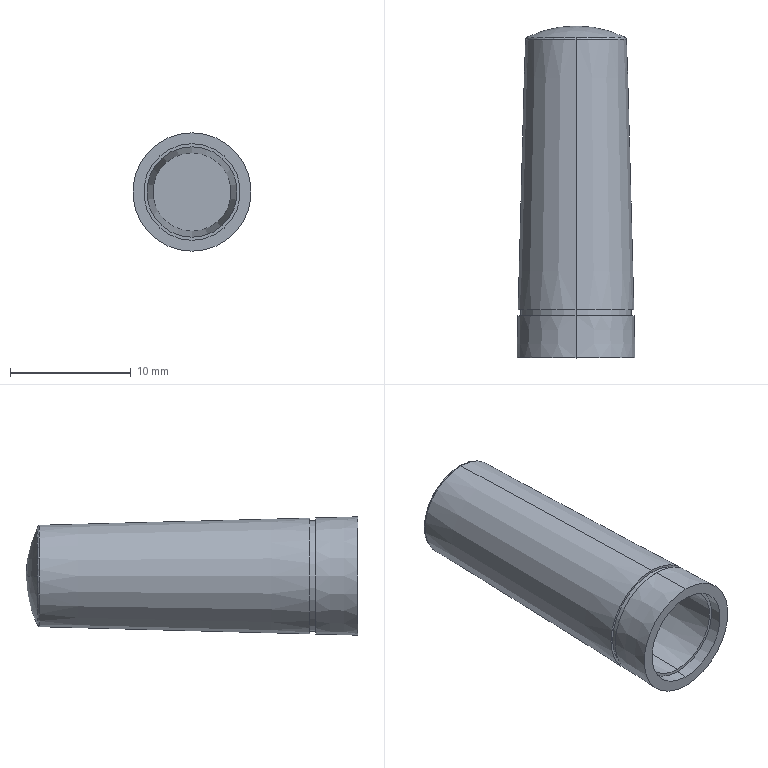Part | SolidWorks | features Revolution 1 | 1 solid | 19 faces | box 9.8 x 27.5 x 9.8 mm | volume 723.478 mm3 | cone 6 | plane 5 | cylinder 4 | sphere 2 | torus 2 | commonest cylinder face diameters 8 x2 9.2 x2
STEP:
#1=CARTESIAN_POINT('',(0.,1.,4.));
#2=VERTEX_POINT('',#1);
#3=CARTESIAN_POINT('',(0.,1.,-4.));
#4=VERTEX_POINT('',#3);
#5=CARTESIAN_POINT('',(0.,1.,0.));
#6=DIRECTION('',(0.,-1.,0.));
#7=DIRECTION('',(0.,0.,-1.));
#8=AXIS2_PLACEMENT_3D('',#5,#6,#7);
#9=CIRCLE('',#8,4.);
#10=EDGE_CURVE('',#2,#4,#9,.T.);
#11=ORIENTED_EDGE('',*,*,#10,.F.);
#12=CARTESIAN_POINT('',(0.,0.,4.));
#13=VERTEX_POINT('',#12);
#14=CARTESIAN_POINT('',(0.,0.,4.));
#15=DIRECTION('',(0.,-1.,0.));
#16=VECTOR('',#15,1000.);
#17=LINE('',#14,#16);
#18=EDGE_CURVE('',#2,#13,#17,.T.);
#19=ORIENTED_EDGE('',*,*,#18,.T.);
#20=CARTESIAN_POINT('',(0.,0.,-4.));
#21=VERTEX_POINT('',#20);
#22=CARTESIAN_POINT('',(0.,0.,0.));
#23=DIRECTION('',(0.,-1.,0.));
#24=DIRECTION('',(0.,0.,-1.));
#25=AXIS2_PLACEMENT_3D('',#22,#23,#24);
#26=CIRCLE('',#25,4.);
#27=EDGE_CURVE('',#13,#21,#26,.T.);
#28=ORIENTED_EDGE('',*,*,#27,.T.);
#29=CARTESIAN_POINT('',(0.,0.,-4.));
#30=DIRECTION('',(0.,-1.,0.));
#31=VECTOR('',#30,1000.);
#32=LINE('',#29,#31);
#33=EDGE_CURVE('',#4,#21,#32,.T.);
#34=ORIENTED_EDGE('',*,*,#33,.F.);
#35=EDGE_LOOP('',(#11,#19,#28,#34));
#36=FACE_OUTER_BOUND('',#35,.T.);
#37=CARTESIAN_POINT('',(0.,0.,0.));
#38=DIRECTION('',(0.,-1.,0.));
#39=DIRECTION('',(0.,0.,-1.));
#40=AXIS2_PLACEMENT_3D('',#37,#38,#39);
#41=CYLINDRICAL_SURFACE('',#40,4.);
#42=ADVANCED_FACE('',(#36),#41,.F.);
#43=CARTESIAN_POINT('',(0.,26.38,3.25));
#44=VERTEX_POINT('',#43);
#45=CARTESIAN_POINT('',(0.,26.38,-3.25));
#46=VERTEX_POINT('',#45);
#47=CARTESIAN_POINT('',(0.,26.38,0.));
#48=DIRECTION('',(0.,-1.,0.));
#49=DIRECTION('',(0.,0.,-1.));
#50=AXIS2_PLACEMENT_3D('',#47,#48,#49);
#51=CIRCLE('',#50,3.25);
#52=EDGE_CURVE('',#44,#46,#51,.T.);
#53=ORIENTED_EDGE('',*,*,#52,.F.);
#54=CARTESIAN_POINT('',(0.,1.,3.75));
#55=VERTEX_POINT('',#54);
#56=CARTESIAN_POINT('',(0.,1.,3.75));
#57=DIRECTION('',(0.,-0.9998,0.0197));
#58=VECTOR('',#57,1000.);
#59=LINE('',#56,#58);
#60=EDGE_CURVE('',#44,#55,#59,.T.);
#61=ORIENTED_EDGE('',*,*,#60,.T.);
#62=CARTESIAN_POINT('',(0.,1.,-3.75));
#63=VERTEX_POINT('',#62);
#64=CARTESIAN_POINT('',(0.,1.,0.));
#65=DIRECTION('',(0.,-1.,0.));
#66=DIRECTION('',(0.,0.,-1.));
#67=AXIS2_PLACEMENT_3D('',#64,#65,#66);
#68=CIRCLE('',#67,3.75);
#69=EDGE_CURVE('',#55,#63,#68,.T.);
#70=ORIENTED_EDGE('',*,*,#69,.T.);
#71=CARTESIAN_POINT('',(0.,1.,-3.75));
#72=DIRECTION('',(0.,-0.9998,-0.0197));
#73=VECTOR('',#72,1000.);
#74=LINE('',#71,#73);
#75=EDGE_CURVE('',#46,#63,#74,.T.);
#76=ORIENTED_EDGE('',*,*,#75,.F.);
#77=EDGE_LOOP('',(#53,#61,#70,#76));
#78=FACE_OUTER_BOUND('',#77,.T.);
#79=CARTESIAN_POINT('',(0.,1.,0.));
#80=DIRECTION('',(0.,-1.,0.));
#81=DIRECTION('',(0.,0.,-1.));
#82=AXIS2_PLACEMENT_3D('',#79,#80,#81);
#83=CONICAL_SURFACE('',#82,3.75,0.0197);
#84=ADVANCED_FACE('',(#78),#83,.F.);
#85=CARTESIAN_POINT('',(0.,27.5,0.));
#86=VERTEX_POINT('',#85);
#87=CARTESIAN_POINT('',(-4.091,26.554,0.));
#88=VERTEX_POINT('',#87);
#89=CARTESIAN_POINT('',(0.,18.18,0.));
#90=DIRECTION('',(0.,0.,1.));
#91=DIRECTION('',(1.,0.,0.));
#92=AXIS2_PLACEMENT_3D('',#89,#90,#91);
#93=CIRCLE('',#92,9.32);
#94=EDGE_CURVE('',#86,#88,#93,.T.);
#95=ORIENTED_EDGE('',*,*,#94,.F.);
#96=CARTESIAN_POINT('',(4.091,26.554,0.));
#97=VERTEX_POINT('',#96);
#98=CARTESIAN_POINT('',(0.,18.18,0.));
#99=DIRECTION('',(0.,0.,-1.));
#100=DIRECTION('',(-1.,0.,0.));
#101=AXIS2_PLACEMENT_3D('',#98,#99,#100);
#102=CIRCLE('',#101,9.32);
#103=EDGE_CURVE('',#86,#97,#102,.T.);
#104=ORIENTED_EDGE('',*,*,#103,.T.);
#105=CARTESIAN_POINT('',(0.,26.554,-4.091));
#106=VERTEX_POINT('',#105);
#107=CARTESIAN_POINT('',(0.,26.554,0.));
#108=DIRECTION('',(0.,-1.,0.));
#109=DIRECTION('',(0.,0.,-1.));
#110=AXIS2_PLACEMENT_3D('',#107,#108,#109);
#111=CIRCLE('',#110,4.091);
#112=EDGE_CURVE('',#106,#97,#111,.T.);
#113=ORIENTED_EDGE('',*,*,#112,.F.);
#114=CARTESIAN_POINT('',(0.,26.554,0.));
#115=DIRECTION('',(0.,-1.,0.));
#116=DIRECTION('',(0.,0.,-1.));
#117=AXIS2_PLACEMENT_3D('',#114,#115,#116);
#118=CIRCLE('',#117,4.091);
#119=EDGE_CURVE('',#88,#106,#118,.T.);
#120=ORIENTED_EDGE('',*,*,#119,.F.);
#121=EDGE_LOOP('',(#95,#104,#113,#120));
#122=FACE_OUTER_BOUND('',#121,.T.);
#123=CARTESIAN_POINT('',(0.,18.18,0.));
#124=DIRECTION('',(0.,0.,-1.));
#125=DIRECTION('',(-1.,0.,0.));
#126=AXIS2_PLACEMENT_3D('',#123,#124,#125);
#127=SPHERICAL_SURFACE('',#126,9.32);
#128=ADVANCED_FACE('',(#122),#127,.T.);
#129=ORIENTED_EDGE('',*,*,#112,.T.);
#130=CARTESIAN_POINT('',(0.,26.554,4.091));
#131=VERTEX_POINT('',#130);
#132=CARTESIAN_POINT('',(0.,26.554,0.));
#133=DIRECTION('',(0.,-1.,0.));
#134=DIRECTION('',(0.,0.,-1.));
#135=AXIS2_PLACEMENT_3D('',#132,#133,#134);
#136=CIRCLE('',#135,4.091);
#137=EDGE_CURVE('',#97,#131,#136,.T.);
#138=ORIENTED_EDGE('',*,*,#137,.T.);
#139=CARTESIAN_POINT('',(0.,26.38,4.203));
#140=VERTEX_POINT('',#139);
#141=CARTESIAN_POINT('',(0.,26.374,4.003));
#142=DIRECTION('',(1.,0.,0.));
#143=DIRECTION('',(0.,0.,-1.));
#144=AXIS2_PLACEMENT_3D('',#141,#142,#143);
#145=CIRCLE('',#144,0.2);
#146=EDGE_CURVE('',#131,#140,#145,.T.);
#147=ORIENTED_EDGE('',*,*,#146,.T.);
#148=CARTESIAN_POINT('',(0.,26.38,-4.203));
#149=VERTEX_POINT('',#148);
#150=CARTESIAN_POINT('',(0.,26.38,0.));
#151=DIRECTION('',(0.,-1.,0.));
#152=DIRECTION('',(0.,0.,-1.));
#153=AXIS2_PLACEMENT_3D('',#150,#151,#152);
#154=CIRCLE('',#153,4.203);
#155=EDGE_CURVE('',#149,#140,#154,.T.);
#156=ORIENTED_EDGE('',*,*,#155,.F.);
#157=CARTESIAN_POINT('',(0.,26.374,-4.003));
#158=DIRECTION('',(-1.,0.,0.));
#159=DIRECTION('',(0.,0.,1.));
#160=AXIS2_PLACEMENT_3D('',#157,#158,#159);
#161=CIRCLE('',#160,0.2);
#162=EDGE_CURVE('',#106,#149,#161,.T.);
#163=ORIENTED_EDGE('',*,*,#162,.F.);
#164=EDGE_LOOP('',(#129,#138,#147,#156,#163));
#165=FACE_OUTER_BOUND('',#164,.T.);
#166=CARTESIAN_POINT('',(0.,26.374,0.));
#167=DIRECTION('',(0.,-1.,0.));
#168=DIRECTION('',(0.,0.,-1.));
#169=AXIS2_PLACEMENT_3D('',#166,#167,#168);
#170=TOROIDAL_SURFACE('',#169,4.003,0.2);
#171=ADVANCED_FACE('',(#165),#170,.T.);
#172=ORIENTED_EDGE('',*,*,#155,.T.);
#173=CARTESIAN_POINT('',(0.,4.,4.794));
#174=VERTEX_POINT('',#173);
#175=CARTESIAN_POINT('',(0.,26.38,4.203));
#176=DIRECTION('',(0.,-0.9997,0.02641));
#177=VECTOR('',#176,1000.);
#178=LINE('',#175,#177);
#179=EDGE_CURVE('',#140,#174,#178,.T.);
#180=ORIENTED_EDGE('',*,*,#179,.T.);
#181=CARTESIAN_POINT('',(0.,4.,-4.794));
#182=VERTEX_POINT('',#181);
#183=CARTESIAN_POINT('',(0.,4.,0.));
#184=DIRECTION('',(0.,-1.,0.));
#185=DIRECTION('',(0.,0.,-1.));
#186=AXIS2_PLACEMENT_3D('',#183,#184,#185);
#187=CIRCLE('',#186,4.794);
#188=EDGE_CURVE('',#182,#174,#187,.T.);
#189=ORIENTED_EDGE('',*,*,#188,.F.);
#190=CARTESIAN_POINT('',(0.,26.38,-4.203));
#191=DIRECTION('',(0.,-0.9997,-0.02641));
#192=VECTOR('',#191,1000.);
#193=LINE('',#190,#192);
#194=EDGE_CURVE('',#149,#182,#193,.T.);
#195=ORIENTED_EDGE('',*,*,#194,.F.);
#196=EDGE_LOOP('',(#172,#180,#189,#195));
#197=FACE_OUTER_BOUND('',#196,.T.);
#198=CARTESIAN_POINT('',(0.,26.38,0.));
#199=DIRECTION('',(0.,-1.,0.));
#200=DIRECTION('',(0.,0.,-1.));
#201=AXIS2_PLACEMENT_3D('',#198,#199,#200);
#202=CONICAL_SURFACE('',#201,4.203,0.02641);
#203=ADVANCED_FACE('',(#197),#202,.T.);
#204=CARTESIAN_POINT('',(0.,4.,-4.6));
#205=VERTEX_POINT('',#204);
#206=CARTESIAN_POINT('',(0.,4.,4.6));
#207=VERTEX_POINT('',#206);
#208=CARTESIAN_POINT('',(0.,4.,0.));
#209=DIRECTION('',(0.,-1.,0.));
#210=DIRECTION('',(0.,0.,-1.));
#211=AXIS2_PLACEMENT_3D('',#208,#209,#210);
#212=CIRCLE('',#211,4.6);
#213=EDGE_CURVE('',#205,#207,#212,.T.);
#214=ORIENTED_EDGE('',*,*,#213,.T.);
#215=CARTESIAN_POINT('',(0.,3.5,4.6));
#216=VERTEX_POINT('',#215);
#217=CARTESIAN_POINT('',(0.,0.,4.6));
#218=DIRECTION('',(0.,-1.,0.));
#219=VECTOR('',#218,1000.);
#220=LINE('',#217,#219);
#221=EDGE_CURVE('',#207,#216,#220,.T.);
#222=ORIENTED_EDGE('',*,*,#221,.T.);
#223=CARTESIAN_POINT('',(0.,3.5,-4.6));
#224=VERTEX_POINT('',#223);
#225=CARTESIAN_POINT('',(0.,3.5,0.));
#226=DIRECTION('',(0.,-1.,0.));
#227=DIRECTION('',(0.,0.,-1.));
#228=AXIS2_PLACEMENT_3D('',#225,#226,#227);
#229=CIRCLE('',#228,4.6);
#230=EDGE_CURVE('',#224,#216,#229,.T.);
#231=ORIENTED_EDGE('',*,*,#230,.F.);
#232=CARTESIAN_POINT('',(0.,0.,-4.6));
#233=DIRECTION('',(0.,-1.,0.));
#234=VECTOR('',#233,1000.);
#235=LINE('',#232,#234);
#236=EDGE_CURVE('',#205,#224,#235,.T.);
#237=ORIENTED_EDGE('',*,*,#236,.F.);
#238=EDGE_LOOP('',(#214,#222,#231,#237));
#239=FACE_OUTER_BOUND('',#238,.T.);
#240=CARTESIAN_POINT('',(0.,0.,0.));
#241=DIRECTION('',(0.,-1.,0.));
#242=DIRECTION('',(0.,0.,-1.));
#243=AXIS2_PLACEMENT_3D('',#240,#241,#242);
#244=CYLINDRICAL_SURFACE('',#243,4.6);
#245=ADVANCED_FACE('',(#239),#244,.T.);
#246=CARTESIAN_POINT('',(0.,3.5,-4.808));
#247=VERTEX_POINT('',#246);
#248=CARTESIAN_POINT('',(0.,3.5,4.808));
#249=VERTEX_POINT('',#248);
#250=CARTESIAN_POINT('',(0.,3.5,0.));
#251=DIRECTION('',(0.,-1.,0.));
#252=DIRECTION('',(0.,0.,-1.));
#253=AXIS2_PLACEMENT_3D('',#250,#251,#252);
#254=CIRCLE('',#253,4.808);
#255=EDGE_CURVE('',#247,#249,#254,.T.);
#256=ORIENTED_EDGE('',*,*,#255,.T.);
#257=CARTESIAN_POINT('',(0.,0.,4.9));
#258=VERTEX_POINT('',#257);
#259=CARTESIAN_POINT('',(0.,3.5,4.808));
#260=DIRECTION('',(0.,-0.9997,0.02641));
#261=VECTOR('',#260,1000.);
#262=LINE('',#259,#261);
#263=EDGE_CURVE('',#249,#258,#262,.T.);
#264=ORIENTED_EDGE('',*,*,#263,.T.);
#265=CARTESIAN_POINT('',(0.,0.,-4.9));
#266=VERTEX_POINT('',#265);
#267=CARTESIAN_POINT('',(0.,0.,0.));
#268=DIRECTION('',(0.,-1.,0.));
#269=DIRECTION('',(0.,0.,-1.));
#270=AXIS2_PLACEMENT_3D('',#267,#268,#269);
#271=CIRCLE('',#270,4.9);
#272=EDGE_CURVE('',#266,#258,#271,.T.);
#273=ORIENTED_EDGE('',*,*,#272,.F.);
#274=CARTESIAN_POINT('',(0.,3.5,-4.808));
#275=DIRECTION('',(0.,-0.9997,-0.02641));
#276=VECTOR('',#275,1000.);
#277=LINE('',#274,#276);
#278=EDGE_CURVE('',#247,#266,#277,.T.);
#279=ORIENTED_EDGE('',*,*,#278,.F.);
#280=EDGE_LOOP('',(#256,#264,#273,#279));
#281=FACE_OUTER_BOUND('',#280,.T.);
#282=CARTESIAN_POINT('',(0.,3.5,0.));
#283=DIRECTION('',(0.,-1.,0.));
#284=DIRECTION('',(0.,0.,-1.));
#285=AXIS2_PLACEMENT_3D('',#282,#283,#284);
#286=CONICAL_SURFACE('',#285,4.808,0.02641);
#287=ADVANCED_FACE('',(#281),#286,.T.);
#288=CARTESIAN_POINT('',(0.,0.,0.));
#289=DIRECTION('',(0.,-1.,0.));
#290=DIRECTION('',(0.,0.,-1.));
#291=AXIS2_PLACEMENT_3D('',#288,#289,#290);
#292=CIRCLE('',#291,4.);
#293=EDGE_CURVE('',#21,#13,#292,.T.);
#294=ORIENTED_EDGE('',*,*,#293,.F.);
#295=ORIENTED_EDGE('',*,*,#27,.F.);
#296=EDGE_LOOP('',(#294,#295));
#297=FACE_BOUND('',#296,.T.);
#298=ORIENTED_EDGE('',*,*,#272,.T.);
#299=CARTESIAN_POINT('',(0.,0.,0.));
#300=DIRECTION('',(0.,-1.,0.));
#301=DIRECTION('',(0.,0.,-1.));
#302=AXIS2_PLACEMENT_3D('',#299,#300,#301);
#303=CIRCLE('',#302,4.9);
#304=EDGE_CURVE('',#258,#266,#303,.T.);
#305=ORIENTED_EDGE('',*,*,#304,.T.);
#306=EDGE_LOOP('',(#298,#305));
#307=FACE_OUTER_BOUND('',#306,.T.);
#308=CARTESIAN_POINT('',(-4.9,0.,0.));
#309=DIRECTION('',(0.,1.,0.));
#310=DIRECTION('',(0.,0.,1.));
#311=AXIS2_PLACEMENT_3D('',#308,#309,#310);
#312=PLANE('',#311);
#313=ADVANCED_FACE('',(#297,#307),#312,.F.);
#314=ORIENTED_EDGE('',*,*,#263,.F.);
#315=CARTESIAN_POINT('',(0.,3.5,0.));
#316=DIRECTION('',(0.,-1.,0.));
#317=DIRECTION('',(0.,0.,-1.));
#318=AXIS2_PLACEMENT_3D('',#315,#316,#317);
#319=CIRCLE('',#318,4.808);
#320=EDGE_CURVE('',#249,#247,#319,.T.);
#321=ORIENTED_EDGE('',*,*,#320,.T.);
#322=ORIENTED_EDGE('',*,*,#278,.T.);
#323=ORIENTED_EDGE('',*,*,#304,.F.);
#324=EDGE_LOOP('',(#314,#321,#322,#323));
#325=FACE_OUTER_BOUND('',#324,.T.);
#326=CARTESIAN_POINT('',(0.,3.5,0.));
#327=DIRECTION('',(0.,-1.,0.));
#328=DIRECTION('',(0.,0.,-1.));
#329=AXIS2_PLACEMENT_3D('',#326,#327,#328);
#330=CONICAL_SURFACE('',#329,4.808,0.02641);
#331=ADVANCED_FACE('',(#325),#330,.T.);
#332=ORIENTED_EDGE('',*,*,#255,.F.);
#333=ORIENTED_EDGE('',*,*,#320,.F.);
#334=EDGE_LOOP('',(#332,#333));
#335=FACE_OUTER_BOUND('',#334,.T.);
#336=ORIENTED_EDGE('',*,*,#230,.T.);
#337=CARTESIAN_POINT('',(0.,3.5,0.));
#338=DIRECTION('',(0.,-1.,0.));
#339=DIRECTION('',(0.,0.,-1.));
#340=AXIS2_PLACEMENT_3D('',#337,#338,#339);
#341=CIRCLE('',#340,4.6);
#342=EDGE_CURVE('',#216,#224,#341,.T.);
#343=ORIENTED_EDGE('',*,*,#342,.T.);
#344=EDGE_LOOP('',(#336,#343));
#345=FACE_BOUND('',#344,.T.);
#346=CARTESIAN_POINT('',(-4.808,3.5,0.));
#347=DIRECTION('',(0.,-1.,0.));
#348=DIRECTION('',(0.,0.,-1.));
#349=AXIS2_PLACEMENT_3D('',#346,#347,#348);
#350=PLANE('',#349);
#351=ADVANCED_FACE('',(#335,#345),#350,.F.);
#352=ORIENTED_EDGE('',*,*,#221,.F.);
#353=CARTESIAN_POINT('',(0.,4.,0.));
#354=DIRECTION('',(0.,-1.,0.));
#355=DIRECTION('',(0.,0.,-1.));
#356=AXIS2_PLACEMENT_3D('',#353,#354,#355);
#357=CIRCLE('',#356,4.6);
#358=EDGE_CURVE('',#207,#205,#357,.T.);
#359=ORIENTED_EDGE('',*,*,#358,.T.);
#360=ORIENTED_EDGE('',*,*,#236,.T.);
#361=ORIENTED_EDGE('',*,*,#342,.F.);
#362=EDGE_LOOP('',(#352,#359,#360,#361));
#363=FACE_OUTER_BOUND('',#362,.T.);
#364=CARTESIAN_POINT('',(0.,0.,0.));
#365=DIRECTION('',(0.,-1.,0.));
#366=DIRECTION('',(0.,0.,-1.));
#367=AXIS2_PLACEMENT_3D('',#364,#365,#366);
#368=CYLINDRICAL_SURFACE('',#367,4.6);
#369=ADVANCED_FACE('',(#363),#368,.T.);
#370=ORIENTED_EDGE('',*,*,#213,.F.);
#371=ORIENTED_EDGE('',*,*,#358,.F.);
#372=EDGE_LOOP('',(#370,#371));
#373=FACE_BOUND('',#372,.T.);
#374=ORIENTED_EDGE('',*,*,#188,.T.);
#375=CARTESIAN_POINT('',(0.,4.,0.));
#376=DIRECTION('',(0.,-1.,0.));
#377=DIRECTION('',(0.,0.,-1.));
#378=AXIS2_PLACEMENT_3D('',#375,#376,#377);
#379=CIRCLE('',#378,4.794);
#380=EDGE_CURVE('',#174,#182,#379,.T.);
#381=ORIENTED_EDGE('',*,*,#380,.T.);
#382=EDGE_LOOP('',(#374,#381));
#383=FACE_OUTER_BOUND('',#382,.T.);
#384=CARTESIAN_POINT('',(-4.6,4.,0.));
#385=DIRECTION('',(0.,1.,0.));
#386=DIRECTION('',(0.,0.,1.));
#387=AXIS2_PLACEMENT_3D('',#384,#385,#386);
#388=PLANE('',#387);
#389=ADVANCED_FACE('',(#373,#383),#388,.F.);
#390=ORIENTED_EDGE('',*,*,#179,.F.);
#391=CARTESIAN_POINT('',(0.,26.38,0.));
#392=DIRECTION('',(0.,-1.,0.));
#393=DIRECTION('',(0.,0.,-1.));
#394=AXIS2_PLACEMENT_3D('',#391,#392,#393);
#395=CIRCLE('',#394,4.203);
#396=EDGE_CURVE('',#140,#149,#395,.T.);
#397=ORIENTED_EDGE('',*,*,#396,.T.);
#398=ORIENTED_EDGE('',*,*,#194,.T.);
#399=ORIENTED_EDGE('',*,*,#380,.F.);
#400=EDGE_LOOP('',(#390,#397,#398,#399));
#401=FACE_OUTER_BOUND('',#400,.T.);
#402=CARTESIAN_POINT('',(0.,26.38,0.));
#403=DIRECTION('',(0.,-1.,0.));
#404=DIRECTION('',(0.,0.,-1.));
#405=AXIS2_PLACEMENT_3D('',#402,#403,#404);
#406=CONICAL_SURFACE('',#405,4.203,0.02641);
#407=ADVANCED_FACE('',(#401),#406,.T.);
#408=ORIENTED_EDGE('',*,*,#146,.F.);
#409=CARTESIAN_POINT('',(0.,26.554,0.));
#410=DIRECTION('',(0.,-1.,0.));
#411=DIRECTION('',(0.,0.,-1.));
#412=AXIS2_PLACEMENT_3D('',#409,#410,#411);
#413=CIRCLE('',#412,4.091);
#414=EDGE_CURVE('',#131,#88,#413,.T.);
#415=ORIENTED_EDGE('',*,*,#414,.T.);
#416=ORIENTED_EDGE('',*,*,#119,.T.);
#417=ORIENTED_EDGE('',*,*,#162,.T.);
#418=ORIENTED_EDGE('',*,*,#396,.F.);
#419=EDGE_LOOP('',(#408,#415,#416,#417,#418));
#420=FACE_OUTER_BOUND('',#419,.T.);
#421=CARTESIAN_POINT('',(0.,26.374,0.));
#422=DIRECTION('',(0.,-1.,0.));
#423=DIRECTION('',(0.,0.,-1.));
#424=AXIS2_PLACEMENT_3D('',#421,#422,#423);
#425=TOROIDAL_SURFACE('',#424,4.003,0.2);
#426=ADVANCED_FACE('',(#420),#425,.T.);
#427=ORIENTED_EDGE('',*,*,#103,.F.);
#428=ORIENTED_EDGE('',*,*,#94,.T.);
#429=ORIENTED_EDGE('',*,*,#414,.F.);
#430=ORIENTED_EDGE('',*,*,#137,.F.);
#431=EDGE_LOOP('',(#427,#428,#429,#430));
#432=FACE_OUTER_BOUND('',#431,.T.);
#433=CARTESIAN_POINT('',(0.,18.18,0.));
#434=DIRECTION('',(0.,0.,-1.));
#435=DIRECTION('',(-1.,0.,0.));
#436=AXIS2_PLACEMENT_3D('',#433,#434,#435);
#437=SPHERICAL_SURFACE('',#436,9.32);
#438=ADVANCED_FACE('',(#432),#437,.T.);
#439=CARTESIAN_POINT('',(0.,26.38,0.));
#440=DIRECTION('',(0.,-1.,0.));
#441=DIRECTION('',(0.,0.,-1.));
#442=AXIS2_PLACEMENT_3D('',#439,#440,#441);
#443=CIRCLE('',#442,3.25);
#444=EDGE_CURVE('',#46,#44,#443,.T.);
#445=ORIENTED_EDGE('',*,*,#444,.T.);
#446=ORIENTED_EDGE('',*,*,#52,.T.);
#447=EDGE_LOOP('',(#445,#446));
#448=FACE_OUTER_BOUND('',#447,.T.);
#449=CARTESIAN_POINT('',(-3.25,26.38,0.));
#450=DIRECTION('',(0.,1.,0.));
#451=DIRECTION('',(0.,0.,1.));
#452=AXIS2_PLACEMENT_3D('',#449,#450,#451);
#453=PLANE('',#452);
#454=ADVANCED_FACE('',(#448),#453,.F.);
#455=ORIENTED_EDGE('',*,*,#60,.F.);
#456=ORIENTED_EDGE('',*,*,#444,.F.);
#457=ORIENTED_EDGE('',*,*,#75,.T.);
#458=CARTESIAN_POINT('',(0.,1.,0.));
#459=DIRECTION('',(0.,-1.,0.));
#460=DIRECTION('',(0.,0.,-1.));
#461=AXIS2_PLACEMENT_3D('',#458,#459,#460);
#462=CIRCLE('',#461,3.75);
#463=EDGE_CURVE('',#63,#55,#462,.T.);
#464=ORIENTED_EDGE('',*,*,#463,.T.);
#465=EDGE_LOOP('',(#455,#456,#457,#464));
#466=FACE_OUTER_BOUND('',#465,.T.);
#467=CARTESIAN_POINT('',(0.,1.,0.));
#468=DIRECTION('',(0.,-1.,0.));
#469=DIRECTION('',(0.,0.,-1.));
#470=AXIS2_PLACEMENT_3D('',#467,#468,#469);
#471=CONICAL_SURFACE('',#470,3.75,0.0197);
#472=ADVANCED_FACE('',(#466),#471,.F.);
#473=ORIENTED_EDGE('',*,*,#463,.F.);
#474=ORIENTED_EDGE('',*,*,#69,.F.);
#475=EDGE_LOOP('',(#473,#474));
#476=FACE_BOUND('',#475,.T.);
#477=CARTESIAN_POINT('',(0.,1.,0.));
#478=DIRECTION('',(0.,-1.,0.));
#479=DIRECTION('',(0.,0.,-1.));
#480=AXIS2_PLACEMENT_3D('',#477,#478,#479);
#481=CIRCLE('',#480,4.);
#482=EDGE_CURVE('',#4,#2,#481,.T.);
#483=ORIENTED_EDGE('',*,*,#482,.T.);
#484=ORIENTED_EDGE('',*,*,#10,.T.);
#485=EDGE_LOOP('',(#483,#484));
#486=FACE_OUTER_BOUND('',#485,.T.);
#487=CARTESIAN_POINT('',(-4.,1.,0.));
#488=DIRECTION('',(0.,1.,0.));
#489=DIRECTION('',(0.,0.,1.));
#490=AXIS2_PLACEMENT_3D('',#487,#488,#489);
#491=PLANE('',#490);
#492=ADVANCED_FACE('',(#476,#486),#491,.F.);
#493=ORIENTED_EDGE('',*,*,#18,.F.);
#494=ORIENTED_EDGE('',*,*,#482,.F.);
#495=ORIENTED_EDGE('',*,*,#33,.T.);
#496=ORIENTED_EDGE('',*,*,#293,.T.);
#497=EDGE_LOOP('',(#493,#494,#495,#496));
#498=FACE_OUTER_BOUND('',#497,.T.);
#499=CARTESIAN_POINT('',(0.,0.,0.));
#500=DIRECTION('',(0.,-1.,0.));
#501=DIRECTION('',(0.,0.,-1.));
#502=AXIS2_PLACEMENT_3D('',#499,#500,#501);
#503=CYLINDRICAL_SURFACE('',#502,4.);
#504=ADVANCED_FACE('',(#498),#503,.F.);
#505=CLOSED_SHELL('',(#42,#84,#128,#171,#203,#245,#287,#313,#331,#351,#369,#389,#407,#426,#438,#454,#472,#492,#504));
#506=MANIFOLD_SOLID_BREP('',#505);
#507=CARTESIAN_POINT('',(0.,0.,0.));
#508=DIRECTION('',(0.,0.,1.));
#509=DIRECTION('',(1.,0.,0.));
#510=AXIS2_PLACEMENT_3D('',#507,#508,#509);
#511=(LENGTH_UNIT()NAMED_UNIT(*)SI_UNIT(.MILLI.,.METRE.));
#512=UNCERTAINTY_MEASURE_WITH_UNIT(LENGTH_MEASURE(0.00001),#511,'','');
#513=(NAMED_UNIT(*)PLANE_ANGLE_UNIT()SI_UNIT($,.RADIAN.));
#514=(NAMED_UNIT(*)SI_UNIT($,.STERADIAN.)SOLID_ANGLE_UNIT());
#515=(GEOMETRIC_REPRESENTATION_CONTEXT(3)GLOBAL_UNCERTAINTY_ASSIGNED_CONTEXT((#512))GLOBAL_UNIT_ASSIGNED_CONTEXT((#511,#513,#514))REPRESENTATION_CONTEXT('',''));
#516=ADVANCED_BREP_SHAPE_REPRESENTATION('',(#506,#510),#515);